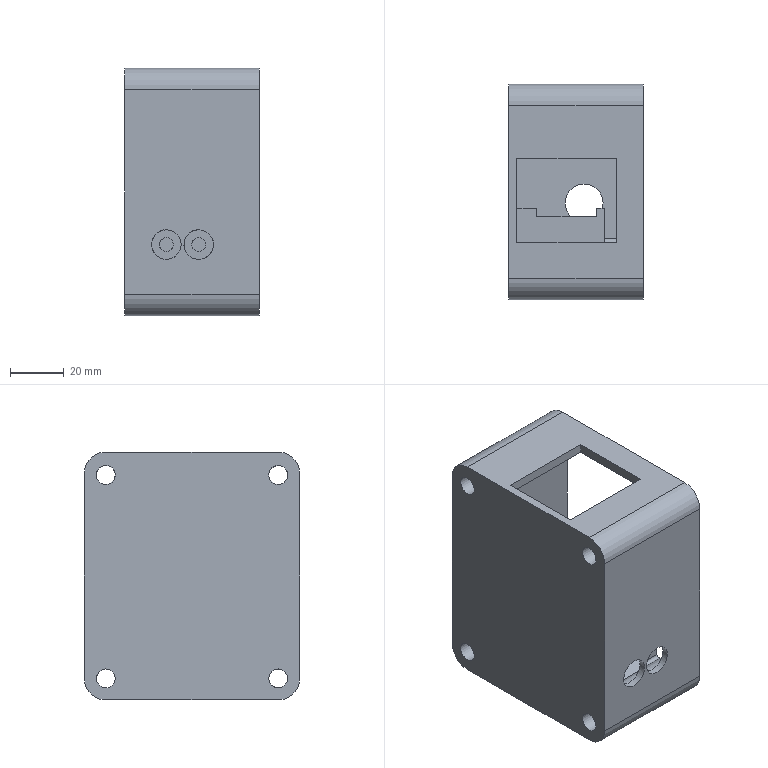Part | 1 solid | 116 faces | box 50 x 80 x 92 mm | volume 112837 mm3 | plane 58 | cylinder 58 | commonest cylinder face diameters 4 x18 1 x6 2.6 x6 6 x6 2 x5 7 x4